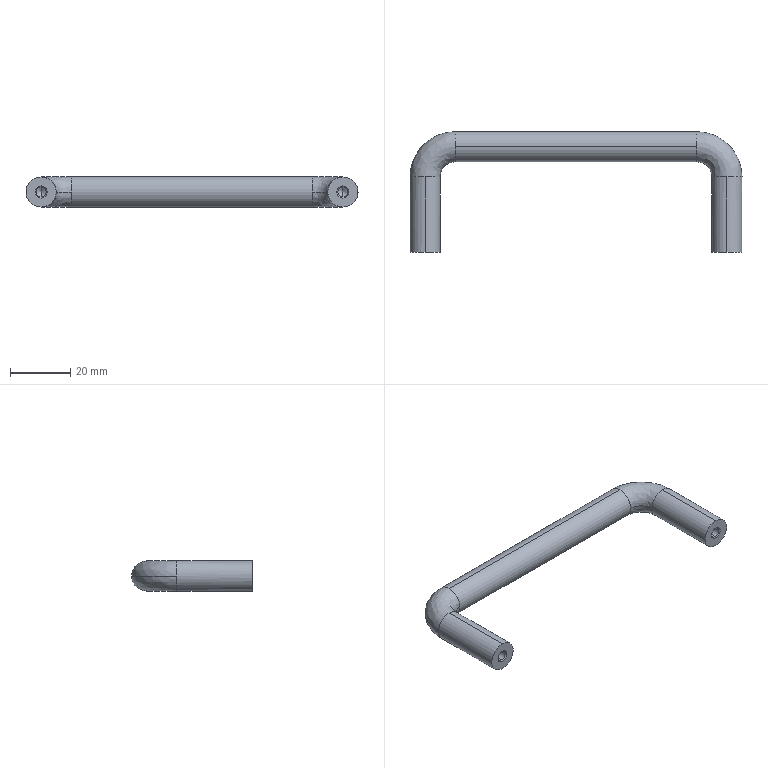Part | SolidWorks | features BaseBody 1 | 1 solid | 24 faces | box 110 x 40 x 10 mm | volume 12474 mm3 | cylinder 10 | cone 8 | spline 4 | plane 2 | commonest cylinder face diameters 10 x6 3.3 x4
STEP:
#1=CARTESIAN_POINT('',(-40.,40.,0.));
#2=VERTEX_POINT('',#1);
#3=CARTESIAN_POINT('',(-40.,35.,5.));
#4=VERTEX_POINT('',#3);
#5=CARTESIAN_POINT('',(-40.,35.,0.));
#6=DIRECTION('',(1.,0.,0.));
#7=DIRECTION('',(0.,0.,-1.));
#8=AXIS2_PLACEMENT_3D('',#5,#6,#7);
#9=CIRCLE('',#8,5.);
#10=EDGE_CURVE('',#2,#4,#9,.T.);
#11=ORIENTED_EDGE('',*,*,#10,.T.);
#12=CARTESIAN_POINT('',(40.,35.,5.));
#13=VERTEX_POINT('',#12);
#14=CARTESIAN_POINT('',(-40.,35.,5.));
#15=DIRECTION('',(1.,0.,0.));
#16=VECTOR('',#15,1000.);
#17=LINE('',#14,#16);
#18=EDGE_CURVE('',#4,#13,#17,.T.);
#19=ORIENTED_EDGE('',*,*,#18,.T.);
#20=CARTESIAN_POINT('',(40.,40.,0.));
#21=VERTEX_POINT('',#20);
#22=CARTESIAN_POINT('',(40.,35.,0.));
#23=DIRECTION('',(-1.,0.,0.));
#24=DIRECTION('',(0.,0.,-1.));
#25=AXIS2_PLACEMENT_3D('',#22,#23,#24);
#26=CIRCLE('',#25,5.);
#27=EDGE_CURVE('',#13,#21,#26,.T.);
#28=ORIENTED_EDGE('',*,*,#27,.T.);
#29=CARTESIAN_POINT('',(40.,35.,-5.));
#30=VERTEX_POINT('',#29);
#31=CARTESIAN_POINT('',(40.,35.,0.));
#32=DIRECTION('',(-1.,0.,0.));
#33=DIRECTION('',(0.,0.,-1.));
#34=AXIS2_PLACEMENT_3D('',#31,#32,#33);
#35=CIRCLE('',#34,5.);
#36=EDGE_CURVE('',#21,#30,#35,.T.);
#37=ORIENTED_EDGE('',*,*,#36,.T.);
#38=CARTESIAN_POINT('',(-40.,35.,-5.));
#39=VERTEX_POINT('',#38);
#40=CARTESIAN_POINT('',(-40.,35.,-5.));
#41=DIRECTION('',(1.,0.,0.));
#42=VECTOR('',#41,1000.);
#43=LINE('',#40,#42);
#44=EDGE_CURVE('',#39,#30,#43,.T.);
#45=ORIENTED_EDGE('',*,*,#44,.F.);
#46=CARTESIAN_POINT('',(-40.,35.,0.));
#47=DIRECTION('',(1.,0.,0.));
#48=DIRECTION('',(0.,0.,-1.));
#49=AXIS2_PLACEMENT_3D('',#46,#47,#48);
#50=CIRCLE('',#49,5.);
#51=EDGE_CURVE('',#39,#2,#50,.T.);
#52=ORIENTED_EDGE('',*,*,#51,.T.);
#53=EDGE_LOOP('',(#11,#19,#28,#37,#45,#52));
#54=FACE_OUTER_BOUND('',#53,.T.);
#55=CARTESIAN_POINT('',(-40.,35.,0.));
#56=DIRECTION('',(1.,0.,0.));
#57=DIRECTION('',(0.,0.,-1.));
#58=AXIS2_PLACEMENT_3D('',#55,#56,#57);
#59=CYLINDRICAL_SURFACE('',#58,5.);
#60=ADVANCED_FACE('',(#54),#59,.T.);
#61=CARTESIAN_POINT('',(40.,30.,0.));
#62=VERTEX_POINT('',#61);
#63=CARTESIAN_POINT('',(40.,35.,0.));
#64=DIRECTION('',(-1.,0.,0.));
#65=DIRECTION('',(0.,0.,-1.));
#66=AXIS2_PLACEMENT_3D('',#63,#64,#65);
#67=CIRCLE('',#66,5.);
#68=EDGE_CURVE('',#62,#13,#67,.T.);
#69=ORIENTED_EDGE('',*,*,#68,.F.);
#70=CARTESIAN_POINT('',(45.,25.,0.));
#71=VERTEX_POINT('',#70);
#72=CARTESIAN_POINT('',(40.,25.,0.));
#73=DIRECTION('',(0.,0.,-1.));
#74=DIRECTION('',(-1.,0.,0.));
#75=AXIS2_PLACEMENT_3D('',#72,#73,#74);
#76=CIRCLE('',#75,5.);
#77=EDGE_CURVE('',#62,#71,#76,.T.);
#78=ORIENTED_EDGE('',*,*,#77,.T.);
#79=CARTESIAN_POINT('',(50.,25.,5.));
#80=VERTEX_POINT('',#79);
#81=CARTESIAN_POINT('',(50.,25.,0.));
#82=DIRECTION('',(0.,1.,0.));
#83=DIRECTION('',(1.,0.,0.));
#84=AXIS2_PLACEMENT_3D('',#81,#82,#83);
#85=CIRCLE('',#84,5.);
#86=EDGE_CURVE('',#71,#80,#85,.T.);
#87=ORIENTED_EDGE('',*,*,#86,.T.);
#88=CARTESIAN_POINT('',(55.,25.,0.));
#89=VERTEX_POINT('',#88);
#90=CARTESIAN_POINT('',(50.,25.,0.));
#91=DIRECTION('',(0.,1.,0.));
#92=DIRECTION('',(1.,0.,0.));
#93=AXIS2_PLACEMENT_3D('',#90,#91,#92);
#94=CIRCLE('',#93,5.);
#95=EDGE_CURVE('',#80,#89,#94,.T.);
#96=ORIENTED_EDGE('',*,*,#95,.T.);
#97=CARTESIAN_POINT('',(40.,25.,0.));
#98=DIRECTION('',(0.,0.,-1.));
#99=DIRECTION('',(-1.,0.,0.));
#100=AXIS2_PLACEMENT_3D('',#97,#98,#99);
#101=CIRCLE('',#100,15.);
#102=EDGE_CURVE('',#21,#89,#101,.T.);
#103=ORIENTED_EDGE('',*,*,#102,.F.);
#104=ORIENTED_EDGE('',*,*,#27,.F.);
#105=EDGE_LOOP('',(#69,#78,#87,#96,#103,#104));
#106=FACE_OUTER_BOUND('',#105,.T.);
#107=CARTESIAN_POINT('',(40.,40.,0.));
#108=CARTESIAN_POINT('',(48.787,40.,0.));
#109=CARTESIAN_POINT('',(55.,33.787,0.));
#110=CARTESIAN_POINT('',(55.,25.,0.));
#111=CARTESIAN_POINT('',(40.,40.,10.));
#112=CARTESIAN_POINT('',(48.787,40.,10.));
#113=CARTESIAN_POINT('',(55.,33.787,10.));
#114=CARTESIAN_POINT('',(55.,25.,10.));
#115=CARTESIAN_POINT('',(40.,30.,10.));
#116=CARTESIAN_POINT('',(42.929,30.,10.));
#117=CARTESIAN_POINT('',(45.,27.929,10.));
#118=CARTESIAN_POINT('',(45.,25.,10.));
#119=CARTESIAN_POINT('',(40.,30.,0.));
#120=CARTESIAN_POINT('',(42.929,30.,0.));
#121=CARTESIAN_POINT('',(45.,27.929,0.));
#122=CARTESIAN_POINT('',(45.,25.,0.));
#123=(BOUNDED_SURFACE()B_SPLINE_SURFACE(3,3,((#107,#108,#109,#110),(#111,#112,#113,#114),(#115,#116,#117,#118),(#119,#120,#121,#122)),.UNSPECIFIED.,.F.,.F.,.F.)B_SPLINE_SURFACE_WITH_KNOTS((4,4),(4,4),(0.,1.),(0.,1.),.UNSPECIFIED.)GEOMETRIC_REPRESENTATION_ITEM()RATIONAL_B_SPLINE_SURFACE(((1.,0.8047,0.8047,1.),(0.3333,0.2682,0.2682,0.3333),(0.3333,0.2682,0.2682,0.3333),(1.,0.8047,0.8047,1.)))REPRESENTATION_ITEM('')SURFACE());
#124=ADVANCED_FACE('',(#106),#123,.T.);
#125=CARTESIAN_POINT('',(-50.,25.,5.));
#126=VERTEX_POINT('',#125);
#127=CARTESIAN_POINT('',(-45.,25.,0.));
#128=VERTEX_POINT('',#127);
#129=CARTESIAN_POINT('',(-50.,25.,0.));
#130=DIRECTION('',(0.,1.,0.));
#131=DIRECTION('',(-1.,0.,0.));
#132=AXIS2_PLACEMENT_3D('',#129,#130,#131);
#133=CIRCLE('',#132,5.);
#134=EDGE_CURVE('',#126,#128,#133,.T.);
#135=ORIENTED_EDGE('',*,*,#134,.T.);
#136=CARTESIAN_POINT('',(-40.,30.,0.));
#137=VERTEX_POINT('',#136);
#138=CARTESIAN_POINT('',(-40.,25.,0.));
#139=DIRECTION('',(0.,0.,-1.));
#140=DIRECTION('',(-1.,0.,0.));
#141=AXIS2_PLACEMENT_3D('',#138,#139,#140);
#142=CIRCLE('',#141,5.);
#143=EDGE_CURVE('',#128,#137,#142,.T.);
#144=ORIENTED_EDGE('',*,*,#143,.T.);
#145=CARTESIAN_POINT('',(-40.,35.,0.));
#146=DIRECTION('',(1.,0.,0.));
#147=DIRECTION('',(0.,0.,-1.));
#148=AXIS2_PLACEMENT_3D('',#145,#146,#147);
#149=CIRCLE('',#148,5.);
#150=EDGE_CURVE('',#4,#137,#149,.T.);
#151=ORIENTED_EDGE('',*,*,#150,.F.);
#152=ORIENTED_EDGE('',*,*,#10,.F.);
#153=CARTESIAN_POINT('',(-55.,25.,0.));
#154=VERTEX_POINT('',#153);
#155=CARTESIAN_POINT('',(-40.,25.,0.));
#156=DIRECTION('',(0.,0.,-1.));
#157=DIRECTION('',(-1.,0.,0.));
#158=AXIS2_PLACEMENT_3D('',#155,#156,#157);
#159=CIRCLE('',#158,15.);
#160=EDGE_CURVE('',#154,#2,#159,.T.);
#161=ORIENTED_EDGE('',*,*,#160,.F.);
#162=CARTESIAN_POINT('',(-50.,25.,0.));
#163=DIRECTION('',(0.,1.,0.));
#164=DIRECTION('',(-1.,0.,0.));
#165=AXIS2_PLACEMENT_3D('',#162,#163,#164);
#166=CIRCLE('',#165,5.);
#167=EDGE_CURVE('',#154,#126,#166,.T.);
#168=ORIENTED_EDGE('',*,*,#167,.T.);
#169=EDGE_LOOP('',(#135,#144,#151,#152,#161,#168));
#170=FACE_OUTER_BOUND('',#169,.T.);
#171=CARTESIAN_POINT('',(-55.,25.,0.));
#172=CARTESIAN_POINT('',(-55.,33.787,0.));
#173=CARTESIAN_POINT('',(-48.787,40.,0.));
#174=CARTESIAN_POINT('',(-40.,40.,0.));
#175=CARTESIAN_POINT('',(-55.,25.,10.));
#176=CARTESIAN_POINT('',(-55.,33.787,10.));
#177=CARTESIAN_POINT('',(-48.787,40.,10.));
#178=CARTESIAN_POINT('',(-40.,40.,10.));
#179=CARTESIAN_POINT('',(-45.,25.,10.));
#180=CARTESIAN_POINT('',(-45.,27.929,10.));
#181=CARTESIAN_POINT('',(-42.929,30.,10.));
#182=CARTESIAN_POINT('',(-40.,30.,10.));
#183=CARTESIAN_POINT('',(-45.,25.,0.));
#184=CARTESIAN_POINT('',(-45.,27.929,0.));
#185=CARTESIAN_POINT('',(-42.929,30.,0.));
#186=CARTESIAN_POINT('',(-40.,30.,0.));
#187=(BOUNDED_SURFACE()B_SPLINE_SURFACE(3,3,((#171,#172,#173,#174),(#175,#176,#177,#178),(#179,#180,#181,#182),(#183,#184,#185,#186)),.UNSPECIFIED.,.F.,.F.,.F.)B_SPLINE_SURFACE_WITH_KNOTS((4,4),(4,4),(0.,1.),(0.,1.),.UNSPECIFIED.)GEOMETRIC_REPRESENTATION_ITEM()RATIONAL_B_SPLINE_SURFACE(((1.,0.8047,0.8047,1.),(0.3333,0.2682,0.2682,0.3333),(0.3333,0.2682,0.2682,0.3333),(1.,0.8047,0.8047,1.)))REPRESENTATION_ITEM('')SURFACE());
#188=ADVANCED_FACE('',(#170),#187,.T.);
#189=ORIENTED_EDGE('',*,*,#95,.F.);
#190=CARTESIAN_POINT('',(50.,0.,5.));
#191=VERTEX_POINT('',#190);
#192=CARTESIAN_POINT('',(50.,25.,5.));
#193=DIRECTION('',(0.,-1.,0.));
#194=VECTOR('',#193,1000.);
#195=LINE('',#192,#194);
#196=EDGE_CURVE('',#80,#191,#195,.T.);
#197=ORIENTED_EDGE('',*,*,#196,.T.);
#198=CARTESIAN_POINT('',(50.,0.,-5.));
#199=VERTEX_POINT('',#198);
#200=CARTESIAN_POINT('',(50.,0.,0.));
#201=DIRECTION('',(0.,1.,0.));
#202=DIRECTION('',(0.,0.,-1.));
#203=AXIS2_PLACEMENT_3D('',#200,#201,#202);
#204=CIRCLE('',#203,5.);
#205=EDGE_CURVE('',#191,#199,#204,.T.);
#206=ORIENTED_EDGE('',*,*,#205,.T.);
#207=CARTESIAN_POINT('',(50.,25.,-5.));
#208=VERTEX_POINT('',#207);
#209=CARTESIAN_POINT('',(50.,25.,-5.));
#210=DIRECTION('',(0.,-1.,0.));
#211=VECTOR('',#210,1000.);
#212=LINE('',#209,#211);
#213=EDGE_CURVE('',#208,#199,#212,.T.);
#214=ORIENTED_EDGE('',*,*,#213,.F.);
#215=CARTESIAN_POINT('',(50.,25.,0.));
#216=DIRECTION('',(0.,1.,0.));
#217=DIRECTION('',(1.,0.,0.));
#218=AXIS2_PLACEMENT_3D('',#215,#216,#217);
#219=CIRCLE('',#218,5.);
#220=EDGE_CURVE('',#89,#208,#219,.T.);
#221=ORIENTED_EDGE('',*,*,#220,.F.);
#222=EDGE_LOOP('',(#189,#197,#206,#214,#221));
#223=FACE_OUTER_BOUND('',#222,.T.);
#224=CARTESIAN_POINT('',(50.,25.,0.));
#225=DIRECTION('',(0.,-1.,0.));
#226=DIRECTION('',(0.,0.,-1.));
#227=AXIS2_PLACEMENT_3D('',#224,#225,#226);
#228=CYLINDRICAL_SURFACE('',#227,5.);
#229=ADVANCED_FACE('',(#223),#228,.T.);
#230=ORIENTED_EDGE('',*,*,#134,.F.);
#231=CARTESIAN_POINT('',(-50.,0.,5.));
#232=VERTEX_POINT('',#231);
#233=CARTESIAN_POINT('',(-50.,25.,5.));
#234=DIRECTION('',(0.,-1.,0.));
#235=VECTOR('',#234,1000.);
#236=LINE('',#233,#235);
#237=EDGE_CURVE('',#126,#232,#236,.T.);
#238=ORIENTED_EDGE('',*,*,#237,.T.);
#239=CARTESIAN_POINT('',(-50.,0.,-5.));
#240=VERTEX_POINT('',#239);
#241=CARTESIAN_POINT('',(-50.,0.,0.));
#242=DIRECTION('',(0.,1.,0.));
#243=DIRECTION('',(0.,0.,-1.));
#244=AXIS2_PLACEMENT_3D('',#241,#242,#243);
#245=CIRCLE('',#244,5.);
#246=EDGE_CURVE('',#232,#240,#245,.T.);
#247=ORIENTED_EDGE('',*,*,#246,.T.);
#248=CARTESIAN_POINT('',(-50.,25.,-5.));
#249=VERTEX_POINT('',#248);
#250=CARTESIAN_POINT('',(-50.,25.,-5.));
#251=DIRECTION('',(0.,-1.,0.));
#252=VECTOR('',#251,1000.);
#253=LINE('',#250,#252);
#254=EDGE_CURVE('',#249,#240,#253,.T.);
#255=ORIENTED_EDGE('',*,*,#254,.F.);
#256=CARTESIAN_POINT('',(-50.,25.,0.));
#257=DIRECTION('',(0.,1.,0.));
#258=DIRECTION('',(-1.,0.,0.));
#259=AXIS2_PLACEMENT_3D('',#256,#257,#258);
#260=CIRCLE('',#259,5.);
#261=EDGE_CURVE('',#128,#249,#260,.T.);
#262=ORIENTED_EDGE('',*,*,#261,.F.);
#263=EDGE_LOOP('',(#230,#238,#247,#255,#262));
#264=FACE_OUTER_BOUND('',#263,.T.);
#265=CARTESIAN_POINT('',(-50.,25.,0.));
#266=DIRECTION('',(0.,-1.,0.));
#267=DIRECTION('',(0.,0.,-1.));
#268=AXIS2_PLACEMENT_3D('',#265,#266,#267);
#269=CYLINDRICAL_SURFACE('',#268,5.);
#270=ADVANCED_FACE('',(#264),#269,.T.);
#271=CARTESIAN_POINT('',(50.,0.375,1.65));
#272=VERTEX_POINT('',#271);
#273=CARTESIAN_POINT('',(50.,0.375,-1.65));
#274=VERTEX_POINT('',#273);
#275=CARTESIAN_POINT('',(50.,0.375,0.));
#276=DIRECTION('',(0.,-1.,0.));
#277=DIRECTION('',(0.,0.,-1.));
#278=AXIS2_PLACEMENT_3D('',#275,#276,#277);
#279=CIRCLE('',#278,1.65);
#280=EDGE_CURVE('',#272,#274,#279,.T.);
#281=ORIENTED_EDGE('',*,*,#280,.F.);
#282=CARTESIAN_POINT('',(50.,0.,2.025));
#283=VERTEX_POINT('',#282);
#284=CARTESIAN_POINT('',(50.,0.,2.025));
#285=DIRECTION('',(0.,-0.7071,0.7071));
#286=VECTOR('',#285,1000.);
#287=LINE('',#284,#286);
#288=EDGE_CURVE('',#272,#283,#287,.T.);
#289=ORIENTED_EDGE('',*,*,#288,.T.);
#290=CARTESIAN_POINT('',(50.,0.,-2.025));
#291=VERTEX_POINT('',#290);
#292=CARTESIAN_POINT('',(50.,0.,0.));
#293=DIRECTION('',(0.,1.,0.));
#294=DIRECTION('',(0.,0.,-1.));
#295=AXIS2_PLACEMENT_3D('',#292,#293,#294);
#296=CIRCLE('',#295,2.025);
#297=EDGE_CURVE('',#291,#283,#296,.T.);
#298=ORIENTED_EDGE('',*,*,#297,.F.);
#299=CARTESIAN_POINT('',(50.,0.,-2.025));
#300=DIRECTION('',(0.,-0.7071,-0.7071));
#301=VECTOR('',#300,1000.);
#302=LINE('',#299,#301);
#303=EDGE_CURVE('',#274,#291,#302,.T.);
#304=ORIENTED_EDGE('',*,*,#303,.F.);
#305=EDGE_LOOP('',(#281,#289,#298,#304));
#306=FACE_OUTER_BOUND('',#305,.T.);
#307=CARTESIAN_POINT('',(50.,0.,0.));
#308=DIRECTION('',(0.,-1.,0.));
#309=DIRECTION('',(0.,0.,-1.));
#310=AXIS2_PLACEMENT_3D('',#307,#308,#309);
#311=CONICAL_SURFACE('',#310,2.025,0.7854);
#312=ADVANCED_FACE('',(#306),#311,.F.);
#313=CARTESIAN_POINT('',(-50.,0.375,1.65));
#314=VERTEX_POINT('',#313);
#315=CARTESIAN_POINT('',(-50.,0.375,-1.65));
#316=VERTEX_POINT('',#315);
#317=CARTESIAN_POINT('',(-50.,0.375,0.));
#318=DIRECTION('',(0.,-1.,0.));
#319=DIRECTION('',(0.,0.,-1.));
#320=AXIS2_PLACEMENT_3D('',#317,#318,#319);
#321=CIRCLE('',#320,1.65);
#322=EDGE_CURVE('',#314,#316,#321,.T.);
#323=ORIENTED_EDGE('',*,*,#322,.F.);
#324=CARTESIAN_POINT('',(-50.,0.,2.025));
#325=VERTEX_POINT('',#324);
#326=CARTESIAN_POINT('',(-50.,0.,2.025));
#327=DIRECTION('',(0.,-0.7071,0.7071));
#328=VECTOR('',#327,1000.);
#329=LINE('',#326,#328);
#330=EDGE_CURVE('',#314,#325,#329,.T.);
#331=ORIENTED_EDGE('',*,*,#330,.T.);
#332=CARTESIAN_POINT('',(-50.,0.,-2.025));
#333=VERTEX_POINT('',#332);
#334=CARTESIAN_POINT('',(-50.,0.,0.));
#335=DIRECTION('',(0.,-1.,0.));
#336=DIRECTION('',(0.,0.,-1.));
#337=AXIS2_PLACEMENT_3D('',#334,#335,#336);
#338=CIRCLE('',#337,2.025);
#339=EDGE_CURVE('',#325,#333,#338,.T.);
#340=ORIENTED_EDGE('',*,*,#339,.T.);
#341=CARTESIAN_POINT('',(-50.,0.,-2.025));
#342=DIRECTION('',(0.,-0.7071,-0.7071));
#343=VECTOR('',#342,1000.);
#344=LINE('',#341,#343);
#345=EDGE_CURVE('',#316,#333,#344,.T.);
#346=ORIENTED_EDGE('',*,*,#345,.F.);
#347=EDGE_LOOP('',(#323,#331,#340,#346));
#348=FACE_OUTER_BOUND('',#347,.T.);
#349=CARTESIAN_POINT('',(-50.,0.,0.));
#350=DIRECTION('',(0.,-1.,0.));
#351=DIRECTION('',(0.,0.,-1.));
#352=AXIS2_PLACEMENT_3D('',#349,#350,#351);
#353=CONICAL_SURFACE('',#352,2.025,0.7854);
#354=ADVANCED_FACE('',(#348),#353,.F.);
#355=CARTESIAN_POINT('',(50.,11.5,1.65));
#356=VERTEX_POINT('',#355);
#357=CARTESIAN_POINT('',(50.,11.5,-1.65));
#358=VERTEX_POINT('',#357);
#359=CARTESIAN_POINT('',(50.,11.5,0.));
#360=DIRECTION('',(0.,-1.,0.));
#361=DIRECTION('',(0.,0.,-1.));
#362=AXIS2_PLACEMENT_3D('',#359,#360,#361);
#363=CIRCLE('',#362,1.65);
#364=EDGE_CURVE('',#356,#358,#363,.T.);
#365=ORIENTED_EDGE('',*,*,#364,.F.);
#366=CARTESIAN_POINT('',(50.,0.,1.65));
#367=DIRECTION('',(0.,-1.,0.));
#368=VECTOR('',#367,1000.);
#369=LINE('',#366,#368);
#370=EDGE_CURVE('',#356,#272,#369,.T.);
#371=ORIENTED_EDGE('',*,*,#370,.T.);
#372=ORIENTED_EDGE('',*,*,#280,.T.);
#373=CARTESIAN_POINT('',(50.,0.,-1.65));
#374=DIRECTION('',(0.,-1.,0.));
#375=VECTOR('',#374,1000.);
#376=LINE('',#373,#375);
#377=EDGE_CURVE('',#358,#274,#376,.T.);
#378=ORIENTED_EDGE('',*,*,#377,.F.);
#379=EDGE_LOOP('',(#365,#371,#372,#378));
#380=FACE_OUTER_BOUND('',#379,.T.);
#381=CARTESIAN_POINT('',(50.,0.,0.));
#382=DIRECTION('',(0.,-1.,0.));
#383=DIRECTION('',(0.,0.,-1.));
#384=AXIS2_PLACEMENT_3D('',#381,#382,#383);
#385=CYLINDRICAL_SURFACE('',#384,1.65);
#386=ADVANCED_FACE('',(#380),#385,.F.);
#387=CARTESIAN_POINT('',(-50.,11.5,1.65));
#388=VERTEX_POINT('',#387);
#389=CARTESIAN_POINT('',(-50.,11.5,-1.65));
#390=VERTEX_POINT('',#389);
#391=CARTESIAN_POINT('',(-50.,11.5,0.));
#392=DIRECTION('',(0.,-1.,0.));
#393=DIRECTION('',(0.,0.,-1.));
#394=AXIS2_PLACEMENT_3D('',#391,#392,#393);
#395=CIRCLE('',#394,1.65);
#396=EDGE_CURVE('',#388,#390,#395,.T.);
#397=ORIENTED_EDGE('',*,*,#396,.F.);
#398=CARTESIAN_POINT('',(-50.,0.,1.65));
#399=DIRECTION('',(0.,-1.,0.));
#400=VECTOR('',#399,1000.);
#401=LINE('',#398,#400);
#402=EDGE_CURVE('',#388,#314,#401,.T.);
#403=ORIENTED_EDGE('',*,*,#402,.T.);
#404=ORIENTED_EDGE('',*,*,#322,.T.);
#405=CARTESIAN_POINT('',(-50.,0.,-1.65));
#406=DIRECTION('',(0.,-1.,0.));
#407=VECTOR('',#406,1000.);
#408=LINE('',#405,#407);
#409=EDGE_CURVE('',#390,#316,#408,.T.);
#410=ORIENTED_EDGE('',*,*,#409,.F.);
#411=EDGE_LOOP('',(#397,#403,#404,#410));
#412=FACE_OUTER_BOUND('',#411,.T.);
#413=CARTESIAN_POINT('',(-50.,0.,0.));
#414=DIRECTION('',(0.,-1.,0.));
#415=DIRECTION('',(0.,0.,-1.));
#416=AXIS2_PLACEMENT_3D('',#413,#414,#415);
#417=CYLINDRICAL_SURFACE('',#416,1.65);
#418=ADVANCED_FACE('',(#412),#417,.F.);
#419=CARTESIAN_POINT('',(50.,12.453,0.));
#420=VERTEX_POINT('',#419);
#421=CARTESIAN_POINT('',(50.,11.5,-1.65));
#422=DIRECTION('',(0.,-0.5,-0.866));
#423=VECTOR('',#422,1000.);
#424=LINE('',#421,#423);
#425=EDGE_CURVE('',#420,#358,#424,.T.);
#426=ORIENTED_EDGE('',*,*,#425,.F.);
#427=CARTESIAN_POINT('',(50.,11.5,1.65));
#428=DIRECTION('',(0.,-0.5,0.866));
#429=VECTOR('',#428,1000.);
#430=LINE('',#427,#429);
#431=EDGE_CURVE('',#420,#356,#430,.T.);
#432=ORIENTED_EDGE('',*,*,#431,.T.);
#433=ORIENTED_EDGE('',*,*,#364,.T.);
#434=EDGE_LOOP('',(#426,#432,#433));
#435=FACE_OUTER_BOUND('',#434,.T.);
#436=CARTESIAN_POINT('',(50.,11.5,0.));
#437=DIRECTION('',(0.,-1.,0.));
#438=DIRECTION('',(0.,0.,-1.));
#439=AXIS2_PLACEMENT_3D('',#436,#437,#438);
#440=CONICAL_SURFACE('',#439,1.65,1.047);
#441=ADVANCED_FACE('',(#435),#440,.F.);
#442=CARTESIAN_POINT('',(-50.,12.453,0.));
#443=VERTEX_POINT('',#442);
#444=CARTESIAN_POINT('',(-50.,11.5,-1.65));
#445=DIRECTION('',(0.,-0.5,-0.866));
#446=VECTOR('',#445,1000.);
#447=LINE('',#444,#446);
#448=EDGE_CURVE('',#443,#390,#447,.T.);
#449=ORIENTED_EDGE('',*,*,#448,.F.);
#450=CARTESIAN_POINT('',(-50.,11.5,1.65));
#451=DIRECTION('',(0.,-0.5,0.866));
#452=VECTOR('',#451,1000.);
#453=LINE('',#450,#452);
#454=EDGE_CURVE('',#443,#388,#453,.T.);
#455=ORIENTED_EDGE('',*,*,#454,.T.);
#456=ORIENTED_EDGE('',*,*,#396,.T.);
#457=EDGE_LOOP('',(#449,#455,#456));
#458=FACE_OUTER_BOUND('',#457,.T.);
#459=CARTESIAN_POINT('',(-50.,11.5,0.));
#460=DIRECTION('',(0.,-1.,0.));
#461=DIRECTION('',(0.,0.,-1.));
#462=AXIS2_PLACEMENT_3D('',#459,#460,#461);
#463=CONICAL_SURFACE('',#462,1.65,1.047);
#464=ADVANCED_FACE('',(#458),#463,.F.);
#465=ORIENTED_EDGE('',*,*,#18,.F.);
#466=ORIENTED_EDGE('',*,*,#150,.T.);
#467=CARTESIAN_POINT('',(-40.,35.,0.));
#468=DIRECTION('',(1.,0.,0.));
#469=DIRECTION('',(0.,0.,-1.));
#470=AXIS2_PLACEMENT_3D('',#467,#468,#469);
#471=CIRCLE('',#470,5.);
#472=EDGE_CURVE('',#137,#39,#471,.T.);
#473=ORIENTED_EDGE('',*,*,#472,.T.);
#474=ORIENTED_EDGE('',*,*,#44,.T.);
#475=CARTESIAN_POINT('',(40.,35.,0.));
#476=DIRECTION('',(-1.,0.,0.));
#477=DIRECTION('',(0.,0.,-1.));
#478=AXIS2_PLACEMENT_3D('',#475,#476,#477);
#479=CIRCLE('',#478,5.);
#480=EDGE_CURVE('',#30,#62,#479,.T.);
#481=ORIENTED_EDGE('',*,*,#480,.T.);
#482=ORIENTED_EDGE('',*,*,#68,.T.);
#483=EDGE_LOOP('',(#465,#466,#473,#474,#481,#482));
#484=FACE_OUTER_BOUND('',#483,.T.);
#485=CARTESIAN_POINT('',(-40.,35.,0.));
#486=DIRECTION('',(1.,0.,0.));
#487=DIRECTION('',(0.,0.,-1.));
#488=AXIS2_PLACEMENT_3D('',#485,#486,#487);
#489=CYLINDRICAL_SURFACE('',#488,5.);
#490=ADVANCED_FACE('',(#484),#489,.T.);
#491=ORIENTED_EDGE('',*,*,#77,.F.);
#492=ORIENTED_EDGE('',*,*,#480,.F.);
#493=ORIENTED_EDGE('',*,*,#36,.F.);
#494=ORIENTED_EDGE('',*,*,#102,.T.);
#495=ORIENTED_EDGE('',*,*,#220,.T.);
#496=CARTESIAN_POINT('',(50.,25.,0.));
#497=DIRECTION('',(0.,1.,0.));
#498=DIRECTION('',(1.,0.,0.));
#499=AXIS2_PLACEMENT_3D('',#496,#497,#498);
#500=CIRCLE('',#499,5.);
#501=EDGE_CURVE('',#208,#71,#500,.T.);
#502=ORIENTED_EDGE('',*,*,#501,.T.);
#503=EDGE_LOOP('',(#491,#492,#493,#494,#495,#502));
#504=FACE_OUTER_BOUND('',#503,.T.);
#505=CARTESIAN_POINT('',(40.,30.,0.));
#506=CARTESIAN_POINT('',(42.929,30.,0.));
#507=CARTESIAN_POINT('',(45.,27.929,0.));
#508=CARTESIAN_POINT('',(45.,25.,0.));
#509=CARTESIAN_POINT('',(40.,30.,-10.));
#510=CARTESIAN_POINT('',(42.929,30.,-10.));
#511=CARTESIAN_POINT('',(45.,27.929,-10.));
#512=CARTESIAN_POINT('',(45.,25.,-10.));
#513=CARTESIAN_POINT('',(40.,40.,-10.));
#514=CARTESIAN_POINT('',(48.787,40.,-10.));
#515=CARTESIAN_POINT('',(55.,33.787,-10.));
#516=CARTESIAN_POINT('',(55.,25.,-10.));
#517=CARTESIAN_POINT('',(40.,40.,0.));
#518=CARTESIAN_POINT('',(48.787,40.,0.));
#519=CARTESIAN_POINT('',(55.,33.787,0.));
#520=CARTESIAN_POINT('',(55.,25.,0.));
#521=(BOUNDED_SURFACE()B_SPLINE_SURFACE(3,3,((#505,#506,#507,#508),(#509,#510,#511,#512),(#513,#514,#515,#516),(#517,#518,#519,#520)),.UNSPECIFIED.,.F.,.F.,.F.)B_SPLINE_SURFACE_WITH_KNOTS((4,4),(4,4),(0.,1.),(0.,1.),.UNSPECIFIED.)GEOMETRIC_REPRESENTATION_ITEM()RATIONAL_B_SPLINE_SURFACE(((1.,0.8047,0.8047,1.),(0.3333,0.2682,0.2682,0.3333),(0.3333,0.2682,0.2682,0.3333),(1.,0.8047,0.8047,1.)))REPRESENTATION_ITEM('')SURFACE());
#522=ADVANCED_FACE('',(#504),#521,.T.);
#523=ORIENTED_EDGE('',*,*,#143,.F.);
#524=ORIENTED_EDGE('',*,*,#261,.T.);
#525=CARTESIAN_POINT('',(-50.,25.,0.));
#526=DIRECTION('',(0.,1.,0.));
#527=DIRECTION('',(-1.,0.,0.));
#528=AXIS2_PLACEMENT_3D('',#525,#526,#527);
#529=CIRCLE('',#528,5.);
#530=EDGE_CURVE('',#249,#154,#529,.T.);
#531=ORIENTED_EDGE('',*,*,#530,.T.);
#532=ORIENTED_EDGE('',*,*,#160,.T.);
#533=ORIENTED_EDGE('',*,*,#51,.F.);
#534=ORIENTED_EDGE('',*,*,#472,.F.);
#535=EDGE_LOOP('',(#523,#524,#531,#532,#533,#534));
#536=FACE_OUTER_BOUND('',#535,.T.);
#537=CARTESIAN_POINT('',(-45.,25.,0.));
#538=CARTESIAN_POINT('',(-45.,27.929,0.));
#539=CARTESIAN_POINT('',(-42.929,30.,0.));
#540=CARTESIAN_POINT('',(-40.,30.,0.));
#541=CARTESIAN_POINT('',(-45.,25.,-10.));
#542=CARTESIAN_POINT('',(-45.,27.929,-10.));
#543=CARTESIAN_POINT('',(-42.929,30.,-10.));
#544=CARTESIAN_POINT('',(-40.,30.,-10.));
#545=CARTESIAN_POINT('',(-55.,25.,-10.));
#546=CARTESIAN_POINT('',(-55.,33.787,-10.));
#547=CARTESIAN_POINT('',(-48.787,40.,-10.));
#548=CARTESIAN_POINT('',(-40.,40.,-10.));
#549=CARTESIAN_POINT('',(-55.,25.,0.));
#550=CARTESIAN_POINT('',(-55.,33.787,0.));
#551=CARTESIAN_POINT('',(-48.787,40.,0.));
#552=CARTESIAN_POINT('',(-40.,40.,0.));
#553=(BOUNDED_SURFACE()B_SPLINE_SURFACE(3,3,((#537,#538,#539,#540),(#541,#542,#543,#544),(#545,#546,#547,#548),(#549,#550,#551,#552)),.UNSPECIFIED.,.F.,.F.,.F.)B_SPLINE_SURFACE_WITH_KNOTS((4,4),(4,4),(0.,1.),(0.,1.),.UNSPECIFIED.)GEOMETRIC_REPRESENTATION_ITEM()RATIONAL_B_SPLINE_SURFACE(((1.,0.8047,0.8047,1.),(0.3333,0.2682,0.2682,0.3333),(0.3333,0.2682,0.2682,0.3333),(1.,0.8047,0.8047,1.)))REPRESENTATION_ITEM('')SURFACE());
#554=ADVANCED_FACE('',(#536),#553,.T.);
#555=ORIENTED_EDGE('',*,*,#196,.F.);
#556=ORIENTED_EDGE('',*,*,#86,.F.);
#557=ORIENTED_EDGE('',*,*,#501,.F.);
#558=ORIENTED_EDGE('',*,*,#213,.T.);
#559=CARTESIAN_POINT('',(50.,0.,0.));
#560=DIRECTION('',(0.,1.,0.));
#561=DIRECTION('',(0.,0.,-1.));
#562=AXIS2_PLACEMENT_3D('',#559,#560,#561);
#563=CIRCLE('',#562,5.);
#564=EDGE_CURVE('',#199,#191,#563,.T.);
#565=ORIENTED_EDGE('',*,*,#564,.T.);
#566=EDGE_LOOP('',(#555,#556,#557,#558,#565));
#567=FACE_OUTER_BOUND('',#566,.T.);
#568=CARTESIAN_POINT('',(50.,25.,0.));
#569=DIRECTION('',(0.,-1.,0.));
#570=DIRECTION('',(0.,0.,-1.));
#571=AXIS2_PLACEMENT_3D('',#568,#569,#570);
#572=CYLINDRICAL_SURFACE('',#571,5.);
#573=ADVANCED_FACE('',(#567),#572,.T.);
#574=ORIENTED_EDGE('',*,*,#237,.F.);
#575=ORIENTED_EDGE('',*,*,#167,.F.);
#576=ORIENTED_EDGE('',*,*,#530,.F.);
#577=ORIENTED_EDGE('',*,*,#254,.T.);
#578=CARTESIAN_POINT('',(-50.,0.,0.));
#579=DIRECTION('',(0.,1.,0.));
#580=DIRECTION('',(0.,0.,-1.));
#581=AXIS2_PLACEMENT_3D('',#578,#579,#580);
#582=CIRCLE('',#581,5.);
#583=EDGE_CURVE('',#240,#232,#582,.T.);
#584=ORIENTED_EDGE('',*,*,#583,.T.);
#585=EDGE_LOOP('',(#574,#575,#576,#577,#584));
#586=FACE_OUTER_BOUND('',#585,.T.);
#587=CARTESIAN_POINT('',(-50.,25.,0.));
#588=DIRECTION('',(0.,-1.,0.));
#589=DIRECTION('',(0.,0.,-1.));
#590=AXIS2_PLACEMENT_3D('',#587,#588,#589);
#591=CYLINDRICAL_SURFACE('',#590,5.);
#592=ADVANCED_FACE('',(#586),#591,.T.);
#593=ORIENTED_EDGE('',*,*,#564,.F.);
#594=ORIENTED_EDGE('',*,*,#205,.F.);
#595=EDGE_LOOP('',(#593,#594));
#596=FACE_OUTER_BOUND('',#595,.T.);
#597=ORIENTED_EDGE('',*,*,#297,.T.);
#598=CARTESIAN_POINT('',(50.,0.,0.));
#599=DIRECTION('',(0.,1.,0.));
#600=DIRECTION('',(0.,0.,-1.));
#601=AXIS2_PLACEMENT_3D('',#598,#599,#600);
#602=CIRCLE('',#601,2.025);
#603=EDGE_CURVE('',#283,#291,#602,.T.);
#604=ORIENTED_EDGE('',*,*,#603,.T.);
#605=EDGE_LOOP('',(#597,#604));
#606=FACE_BOUND('',#605,.T.);
#607=CARTESIAN_POINT('',(50.,0.,0.));
#608=DIRECTION('',(0.,-1.,0.));
#609=DIRECTION('',(1.,0.,0.));
#610=AXIS2_PLACEMENT_3D('',#607,#608,#609);
#611=PLANE('',#610);
#612=ADVANCED_FACE('',(#596,#606),#611,.T.);
#613=ORIENTED_EDGE('',*,*,#583,.F.);
#614=ORIENTED_EDGE('',*,*,#246,.F.);
#615=EDGE_LOOP('',(#613,#614));
#616=FACE_OUTER_BOUND('',#615,.T.);
#617=CARTESIAN_POINT('',(-50.,0.,0.));
#618=DIRECTION('',(0.,-1.,0.));
#619=DIRECTION('',(0.,0.,-1.));
#620=AXIS2_PLACEMENT_3D('',#617,#618,#619);
#621=CIRCLE('',#620,2.025);
#622=EDGE_CURVE('',#333,#325,#621,.T.);
#623=ORIENTED_EDGE('',*,*,#622,.F.);
#624=ORIENTED_EDGE('',*,*,#339,.F.);
#625=EDGE_LOOP('',(#623,#624));
#626=FACE_BOUND('',#625,.T.);
#627=CARTESIAN_POINT('',(-50.,0.,0.));
#628=DIRECTION('',(0.,1.,0.));
#629=DIRECTION('',(0.,0.,1.));
#630=AXIS2_PLACEMENT_3D('',#627,#628,#629);
#631=PLANE('',#630);
#632=ADVANCED_FACE('',(#616,#626),#631,.F.);
#633=ORIENTED_EDGE('',*,*,#288,.F.);
#634=CARTESIAN_POINT('',(50.,0.375,0.));
#635=DIRECTION('',(0.,-1.,0.));
#636=DIRECTION('',(0.,0.,-1.));
#637=AXIS2_PLACEMENT_3D('',#634,#635,#636);
#638=CIRCLE('',#637,1.65);
#639=EDGE_CURVE('',#274,#272,#638,.T.);
#640=ORIENTED_EDGE('',*,*,#639,.F.);
#641=ORIENTED_EDGE('',*,*,#303,.T.);
#642=ORIENTED_EDGE('',*,*,#603,.F.);
#643=EDGE_LOOP('',(#633,#640,#641,#642));
#644=FACE_OUTER_BOUND('',#643,.T.);
#645=CARTESIAN_POINT('',(50.,0.,0.));
#646=DIRECTION('',(0.,-1.,0.));
#647=DIRECTION('',(0.,0.,-1.));
#648=AXIS2_PLACEMENT_3D('',#645,#646,#647);
#649=CONICAL_SURFACE('',#648,2.025,0.7854);
#650=ADVANCED_FACE('',(#644),#649,.F.);
#651=ORIENTED_EDGE('',*,*,#330,.F.);
#652=CARTESIAN_POINT('',(-50.,0.375,0.));
#653=DIRECTION('',(0.,-1.,0.));
#654=DIRECTION('',(0.,0.,-1.));
#655=AXIS2_PLACEMENT_3D('',#652,#653,#654);
#656=CIRCLE('',#655,1.65);
#657=EDGE_CURVE('',#316,#314,#656,.T.);
#658=ORIENTED_EDGE('',*,*,#657,.F.);
#659=ORIENTED_EDGE('',*,*,#345,.T.);
#660=ORIENTED_EDGE('',*,*,#622,.T.);
#661=EDGE_LOOP('',(#651,#658,#659,#660));
#662=FACE_OUTER_BOUND('',#661,.T.);
#663=CARTESIAN_POINT('',(-50.,0.,0.));
#664=DIRECTION('',(0.,-1.,0.));
#665=DIRECTION('',(0.,0.,-1.));
#666=AXIS2_PLACEMENT_3D('',#663,#664,#665);
#667=CONICAL_SURFACE('',#666,2.025,0.7854);
#668=ADVANCED_FACE('',(#662),#667,.F.);
#669=ORIENTED_EDGE('',*,*,#370,.F.);
#670=CARTESIAN_POINT('',(50.,11.5,0.));
#671=DIRECTION('',(0.,-1.,0.));
#672=DIRECTION('',(0.,0.,-1.));
#673=AXIS2_PLACEMENT_3D('',#670,#671,#672);
#674=CIRCLE('',#673,1.65);
#675=EDGE_CURVE('',#358,#356,#674,.T.);
#676=ORIENTED_EDGE('',*,*,#675,.F.);
#677=ORIENTED_EDGE('',*,*,#377,.T.);
#678=ORIENTED_EDGE('',*,*,#639,.T.);
#679=EDGE_LOOP('',(#669,#676,#677,#678));
#680=FACE_OUTER_BOUND('',#679,.T.);
#681=CARTESIAN_POINT('',(50.,0.,0.));
#682=DIRECTION('',(0.,-1.,0.));
#683=DIRECTION('',(0.,0.,-1.));
#684=AXIS2_PLACEMENT_3D('',#681,#682,#683);
#685=CYLINDRICAL_SURFACE('',#684,1.65);
#686=ADVANCED_FACE('',(#680),#685,.F.);
#687=ORIENTED_EDGE('',*,*,#402,.F.);
#688=CARTESIAN_POINT('',(-50.,11.5,0.));
#689=DIRECTION('',(0.,-1.,0.));
#690=DIRECTION('',(0.,0.,-1.));
#691=AXIS2_PLACEMENT_3D('',#688,#689,#690);
#692=CIRCLE('',#691,1.65);
#693=EDGE_CURVE('',#390,#388,#692,.T.);
#694=ORIENTED_EDGE('',*,*,#693,.F.);
#695=ORIENTED_EDGE('',*,*,#409,.T.);
#696=ORIENTED_EDGE('',*,*,#657,.T.);
#697=EDGE_LOOP('',(#687,#694,#695,#696));
#698=FACE_OUTER_BOUND('',#697,.T.);
#699=CARTESIAN_POINT('',(-50.,0.,0.));
#700=DIRECTION('',(0.,-1.,0.));
#701=DIRECTION('',(0.,0.,-1.));
#702=AXIS2_PLACEMENT_3D('',#699,#700,#701);
#703=CYLINDRICAL_SURFACE('',#702,1.65);
#704=ADVANCED_FACE('',(#698),#703,.F.);
#705=ORIENTED_EDGE('',*,*,#431,.F.);
#706=ORIENTED_EDGE('',*,*,#425,.T.);
#707=ORIENTED_EDGE('',*,*,#675,.T.);
#708=EDGE_LOOP('',(#705,#706,#707));
#709=FACE_OUTER_BOUND('',#708,.T.);
#710=CARTESIAN_POINT('',(50.,11.5,0.));
#711=DIRECTION('',(0.,-1.,0.));
#712=DIRECTION('',(0.,0.,-1.));
#713=AXIS2_PLACEMENT_3D('',#710,#711,#712);
#714=CONICAL_SURFACE('',#713,1.65,1.047);
#715=ADVANCED_FACE('',(#709),#714,.F.);
#716=ORIENTED_EDGE('',*,*,#454,.F.);
#717=ORIENTED_EDGE('',*,*,#448,.T.);
#718=ORIENTED_EDGE('',*,*,#693,.T.);
#719=EDGE_LOOP('',(#716,#717,#718));
#720=FACE_OUTER_BOUND('',#719,.T.);
#721=CARTESIAN_POINT('',(-50.,11.5,0.));
#722=DIRECTION('',(0.,-1.,0.));
#723=DIRECTION('',(0.,0.,-1.));
#724=AXIS2_PLACEMENT_3D('',#721,#722,#723);
#725=CONICAL_SURFACE('',#724,1.65,1.047);
#726=ADVANCED_FACE('',(#720),#725,.F.);
#727=CLOSED_SHELL('',(#60,#124,#188,#229,#270,#312,#354,#386,#418,#441,#464,#490,#522,#554,#573,#592,#612,#632,#650,#668,#686,#704,#715,#726));
#728=MANIFOLD_SOLID_BREP('',#727);
#729=CARTESIAN_POINT('',(0.,0.,0.));
#730=DIRECTION('',(0.,0.,1.));
#731=DIRECTION('',(1.,0.,0.));
#732=AXIS2_PLACEMENT_3D('',#729,#730,#731);
#733=(LENGTH_UNIT()NAMED_UNIT(*)SI_UNIT(.MILLI.,.METRE.));
#734=UNCERTAINTY_MEASURE_WITH_UNIT(LENGTH_MEASURE(0.00001),#733,'','');
#735=(NAMED_UNIT(*)PLANE_ANGLE_UNIT()SI_UNIT($,.RADIAN.));
#736=(NAMED_UNIT(*)SI_UNIT($,.STERADIAN.)SOLID_ANGLE_UNIT());
#737=(GEOMETRIC_REPRESENTATION_CONTEXT(3)GLOBAL_UNCERTAINTY_ASSIGNED_CONTEXT((#734))GLOBAL_UNIT_ASSIGNED_CONTEXT((#733,#735,#736))REPRESENTATION_CONTEXT('',''));
#738=ADVANCED_BREP_SHAPE_REPRESENTATION('',(#728,#732),#737);